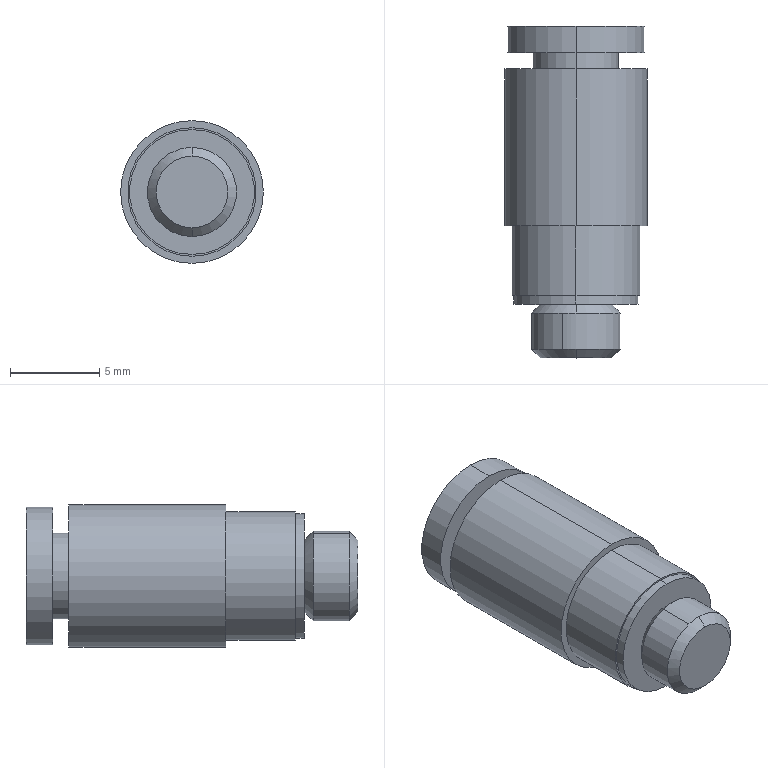Part | SolidWorks | features BaseBody 1 | 1 solid | 33 faces | box 8 x 18.6 x 8 mm | volume 570.386 mm3 | plane 15 | cylinder 14 | cone 4 | commonest cylinder face diameters 4 x2 4.8 x2 5 x2 7 x2 7.2 x2 7.7 x2
STEP:
#1=CARTESIAN_POINT('',(0.,15.6,3.85));
#2=VERTEX_POINT('',#1);
#3=CARTESIAN_POINT('',(0.,15.6,-3.85));
#4=VERTEX_POINT('',#3);
#5=CARTESIAN_POINT('',(0.,15.6,0.));
#6=DIRECTION('',(0.,-1.,0.));
#7=DIRECTION('',(0.,0.,-1.));
#8=AXIS2_PLACEMENT_3D('',#5,#6,#7);
#9=CIRCLE('',#8,3.85);
#10=EDGE_CURVE('',#2,#4,#9,.T.);
#11=ORIENTED_EDGE('',*,*,#10,.F.);
#12=CARTESIAN_POINT('',(0.,15.6,0.));
#13=DIRECTION('',(0.,-1.,0.));
#14=DIRECTION('',(0.,0.,-1.));
#15=AXIS2_PLACEMENT_3D('',#12,#13,#14);
#16=CIRCLE('',#15,3.85);
#17=EDGE_CURVE('',#4,#2,#16,.T.);
#18=ORIENTED_EDGE('',*,*,#17,.F.);
#19=EDGE_LOOP('',(#11,#18));
#20=FACE_OUTER_BOUND('',#19,.T.);
#21=CARTESIAN_POINT('',(0.,15.6,-2.));
#22=VERTEX_POINT('',#21);
#23=CARTESIAN_POINT('',(0.,15.6,2.));
#24=VERTEX_POINT('',#23);
#25=CARTESIAN_POINT('',(0.,15.6,0.));
#26=DIRECTION('',(0.,-1.,0.));
#27=DIRECTION('',(0.,0.,-1.));
#28=AXIS2_PLACEMENT_3D('',#25,#26,#27);
#29=CIRCLE('',#28,2.);
#30=EDGE_CURVE('',#22,#24,#29,.T.);
#31=ORIENTED_EDGE('',*,*,#30,.T.);
#32=CARTESIAN_POINT('',(0.,15.6,0.));
#33=DIRECTION('',(0.,-1.,0.));
#34=DIRECTION('',(0.,0.,-1.));
#35=AXIS2_PLACEMENT_3D('',#32,#33,#34);
#36=CIRCLE('',#35,2.);
#37=EDGE_CURVE('',#24,#22,#36,.T.);
#38=ORIENTED_EDGE('',*,*,#37,.T.);
#39=EDGE_LOOP('',(#31,#38));
#40=FACE_BOUND('',#39,.T.);
#41=CARTESIAN_POINT('',(0.,15.6,0.));
#42=DIRECTION('',(0.,-1.,0.));
#43=DIRECTION('',(0.,0.,-1.));
#44=AXIS2_PLACEMENT_3D('',#41,#42,#43);
#45=PLANE('',#44);
#46=ADVANCED_FACE('',(#20,#40),#45,.F.);
#47=CARTESIAN_POINT('',(0.,2.3,2.));
#48=VERTEX_POINT('',#47);
#49=CARTESIAN_POINT('',(0.,15.6,2.));
#50=DIRECTION('',(0.,-1.,0.));
#51=VECTOR('',#50,1000.);
#52=LINE('',#49,#51);
#53=EDGE_CURVE('',#24,#48,#52,.T.);
#54=ORIENTED_EDGE('',*,*,#53,.T.);
#55=CARTESIAN_POINT('',(0.,2.3,-2.));
#56=VERTEX_POINT('',#55);
#57=CARTESIAN_POINT('',(0.,2.3,0.));
#58=DIRECTION('',(0.,-1.,0.));
#59=DIRECTION('',(0.,0.,-1.));
#60=AXIS2_PLACEMENT_3D('',#57,#58,#59);
#61=CIRCLE('',#60,2.);
#62=EDGE_CURVE('',#48,#56,#61,.T.);
#63=ORIENTED_EDGE('',*,*,#62,.T.);
#64=CARTESIAN_POINT('',(0.,15.6,-2.));
#65=DIRECTION('',(0.,-1.,0.));
#66=VECTOR('',#65,1000.);
#67=LINE('',#64,#66);
#68=EDGE_CURVE('',#22,#56,#67,.T.);
#69=ORIENTED_EDGE('',*,*,#68,.F.);
#70=ORIENTED_EDGE('',*,*,#37,.F.);
#71=EDGE_LOOP('',(#54,#63,#69,#70));
#72=FACE_OUTER_BOUND('',#71,.T.);
#73=CARTESIAN_POINT('',(0.,2.3,0.));
#74=DIRECTION('',(0.,-1.,0.));
#75=DIRECTION('',(1.,0.,0.));
#76=AXIS2_PLACEMENT_3D('',#73,#74,#75);
#77=CYLINDRICAL_SURFACE('',#76,2.);
#78=ADVANCED_FACE('',(#72),#77,.F.);
#79=ORIENTED_EDGE('',*,*,#53,.F.);
#80=ORIENTED_EDGE('',*,*,#30,.F.);
#81=ORIENTED_EDGE('',*,*,#68,.T.);
#82=CARTESIAN_POINT('',(0.,2.3,0.));
#83=DIRECTION('',(0.,-1.,0.));
#84=DIRECTION('',(0.,0.,-1.));
#85=AXIS2_PLACEMENT_3D('',#82,#83,#84);
#86=CIRCLE('',#85,2.);
#87=EDGE_CURVE('',#56,#48,#86,.T.);
#88=ORIENTED_EDGE('',*,*,#87,.T.);
#89=EDGE_LOOP('',(#79,#80,#81,#88));
#90=FACE_OUTER_BOUND('',#89,.T.);
#91=CARTESIAN_POINT('',(0.,2.3,0.));
#92=DIRECTION('',(0.,-1.,0.));
#93=DIRECTION('',(-1.,0.,0.));
#94=AXIS2_PLACEMENT_3D('',#91,#92,#93);
#95=CYLINDRICAL_SURFACE('',#94,2.);
#96=ADVANCED_FACE('',(#90),#95,.F.);
#97=CARTESIAN_POINT('',(1.25,2.3,0.7217));
#98=VERTEX_POINT('',#97);
#99=CARTESIAN_POINT('',(1.25,2.3,-0.7217));
#100=VERTEX_POINT('',#99);
#101=CARTESIAN_POINT('',(1.25,2.3,0.));
#102=DIRECTION('',(0.,0.,-1.));
#103=VECTOR('',#102,1000.);
#104=LINE('',#101,#103);
#105=EDGE_CURVE('',#98,#100,#104,.T.);
#106=ORIENTED_EDGE('',*,*,#105,.F.);
#107=CARTESIAN_POINT('',(0.,2.3,1.443));
#108=VERTEX_POINT('',#107);
#109=CARTESIAN_POINT('',(2.125,2.3,0.2165));
#110=DIRECTION('',(0.866,0.,-0.5));
#111=VECTOR('',#110,1000.);
#112=LINE('',#109,#111);
#113=EDGE_CURVE('',#108,#98,#112,.T.);
#114=ORIENTED_EDGE('',*,*,#113,.F.);
#115=CARTESIAN_POINT('',(-1.25,2.3,0.7217));
#116=VERTEX_POINT('',#115);
#117=CARTESIAN_POINT('',(0.875,2.3,1.949));
#118=DIRECTION('',(0.866,0.,0.5));
#119=VECTOR('',#118,1000.);
#120=LINE('',#117,#119);
#121=EDGE_CURVE('',#116,#108,#120,.T.);
#122=ORIENTED_EDGE('',*,*,#121,.F.);
#123=CARTESIAN_POINT('',(-1.25,2.3,-0.7217));
#124=VERTEX_POINT('',#123);
#125=CARTESIAN_POINT('',(-1.25,2.3,0.));
#126=DIRECTION('',(0.,0.,1.));
#127=VECTOR('',#126,1000.);
#128=LINE('',#125,#127);
#129=EDGE_CURVE('',#124,#116,#128,.T.);
#130=ORIENTED_EDGE('',*,*,#129,.F.);
#131=CARTESIAN_POINT('',(0.,2.3,-1.443));
#132=VERTEX_POINT('',#131);
#133=CARTESIAN_POINT('',(0.875,2.3,-1.949));
#134=DIRECTION('',(-0.866,0.,0.5));
#135=VECTOR('',#134,1000.);
#136=LINE('',#133,#135);
#137=EDGE_CURVE('',#132,#124,#136,.T.);
#138=ORIENTED_EDGE('',*,*,#137,.F.);
#139=CARTESIAN_POINT('',(2.125,2.3,-0.2165));
#140=DIRECTION('',(-0.866,0.,-0.5));
#141=VECTOR('',#140,1000.);
#142=LINE('',#139,#141);
#143=EDGE_CURVE('',#100,#132,#142,.T.);
#144=ORIENTED_EDGE('',*,*,#143,.F.);
#145=EDGE_LOOP('',(#106,#114,#122,#130,#138,#144));
#146=FACE_BOUND('',#145,.T.);
#147=ORIENTED_EDGE('',*,*,#62,.F.);
#148=ORIENTED_EDGE('',*,*,#87,.F.);
#149=EDGE_LOOP('',(#147,#148));
#150=FACE_OUTER_BOUND('',#149,.T.);
#151=CARTESIAN_POINT('',(2.,2.3,0.));
#152=DIRECTION('',(0.,1.,0.));
#153=DIRECTION('',(0.,0.,1.));
#154=AXIS2_PLACEMENT_3D('',#151,#152,#153);
#155=PLANE('',#154);
#156=ADVANCED_FACE('',(#146,#150),#155,.T.);
#157=ORIENTED_EDGE('',*,*,#143,.T.);
#158=CARTESIAN_POINT('',(0.,-2.2,-1.443));
#159=VERTEX_POINT('',#158);
#160=CARTESIAN_POINT('',(0.,-2.2,-1.443));
#161=DIRECTION('',(0.,1.,0.));
#162=VECTOR('',#161,1000.);
#163=LINE('',#160,#162);
#164=EDGE_CURVE('',#159,#132,#163,.T.);
#165=ORIENTED_EDGE('',*,*,#164,.F.);
#166=CARTESIAN_POINT('',(1.25,-2.2,-0.7217));
#167=VERTEX_POINT('',#166);
#168=CARTESIAN_POINT('',(1.25,-2.2,-0.7217));
#169=DIRECTION('',(-0.866,0.,-0.5));
#170=VECTOR('',#169,1000.);
#171=LINE('',#168,#170);
#172=EDGE_CURVE('',#167,#159,#171,.T.);
#173=ORIENTED_EDGE('',*,*,#172,.F.);
#174=CARTESIAN_POINT('',(1.25,-2.2,-0.7217));
#175=DIRECTION('',(0.,1.,0.));
#176=VECTOR('',#175,1000.);
#177=LINE('',#174,#176);
#178=EDGE_CURVE('',#167,#100,#177,.T.);
#179=ORIENTED_EDGE('',*,*,#178,.T.);
#180=EDGE_LOOP('',(#157,#165,#173,#179));
#181=FACE_OUTER_BOUND('',#180,.T.);
#182=CARTESIAN_POINT('',(1.25,-2.2,-0.7217));
#183=DIRECTION('',(0.5,0.,-0.866));
#184=DIRECTION('',(-0.866,0.,-0.5));
#185=AXIS2_PLACEMENT_3D('',#182,#183,#184);
#186=PLANE('',#185);
#187=ADVANCED_FACE('',(#181),#186,.F.);
#188=CARTESIAN_POINT('',(1.25,-2.2,0.7217));
#189=VERTEX_POINT('',#188);
#190=CARTESIAN_POINT('',(1.25,-2.2,0.7217));
#191=DIRECTION('',(0.,1.,0.));
#192=VECTOR('',#191,1000.);
#193=LINE('',#190,#192);
#194=EDGE_CURVE('',#189,#98,#193,.T.);
#195=ORIENTED_EDGE('',*,*,#194,.T.);
#196=ORIENTED_EDGE('',*,*,#105,.T.);
#197=ORIENTED_EDGE('',*,*,#178,.F.);
#198=CARTESIAN_POINT('',(1.25,-2.2,0.7217));
#199=DIRECTION('',(0.,0.,-1.));
#200=VECTOR('',#199,1000.);
#201=LINE('',#198,#200);
#202=EDGE_CURVE('',#189,#167,#201,.T.);
#203=ORIENTED_EDGE('',*,*,#202,.F.);
#204=EDGE_LOOP('',(#195,#196,#197,#203));
#205=FACE_OUTER_BOUND('',#204,.T.);
#206=CARTESIAN_POINT('',(1.25,-2.2,0.7217));
#207=DIRECTION('',(1.,0.,0.));
#208=DIRECTION('',(0.,0.,-1.));
#209=AXIS2_PLACEMENT_3D('',#206,#207,#208);
#210=PLANE('',#209);
#211=ADVANCED_FACE('',(#205),#210,.F.);
#212=CARTESIAN_POINT('',(-1.25,-2.2,-0.7217));
#213=VERTEX_POINT('',#212);
#214=CARTESIAN_POINT('',(-1.25,-2.2,0.7217));
#215=VERTEX_POINT('',#214);
#216=CARTESIAN_POINT('',(-1.25,-2.2,-0.7217));
#217=DIRECTION('',(0.,0.,1.));
#218=VECTOR('',#217,1000.);
#219=LINE('',#216,#218);
#220=EDGE_CURVE('',#213,#215,#219,.T.);
#221=ORIENTED_EDGE('',*,*,#220,.T.);
#222=CARTESIAN_POINT('',(0.,-2.2,1.443));
#223=VERTEX_POINT('',#222);
#224=CARTESIAN_POINT('',(-1.25,-2.2,0.7217));
#225=DIRECTION('',(0.866,0.,0.5));
#226=VECTOR('',#225,1000.);
#227=LINE('',#224,#226);
#228=EDGE_CURVE('',#215,#223,#227,.T.);
#229=ORIENTED_EDGE('',*,*,#228,.T.);
#230=CARTESIAN_POINT('',(0.,-2.2,1.443));
#231=DIRECTION('',(0.866,0.,-0.5));
#232=VECTOR('',#231,1000.);
#233=LINE('',#230,#232);
#234=EDGE_CURVE('',#223,#189,#233,.T.);
#235=ORIENTED_EDGE('',*,*,#234,.T.);
#236=ORIENTED_EDGE('',*,*,#202,.T.);
#237=ORIENTED_EDGE('',*,*,#172,.T.);
#238=CARTESIAN_POINT('',(0.,-2.2,-1.443));
#239=DIRECTION('',(-0.866,0.,0.5));
#240=VECTOR('',#239,1000.);
#241=LINE('',#238,#240);
#242=EDGE_CURVE('',#159,#213,#241,.T.);
#243=ORIENTED_EDGE('',*,*,#242,.T.);
#244=EDGE_LOOP('',(#221,#229,#235,#236,#237,#243));
#245=FACE_OUTER_BOUND('',#244,.T.);
#246=CARTESIAN_POINT('',(0.,-2.2,0.));
#247=DIRECTION('',(0.,1.,0.));
#248=DIRECTION('',(0.,0.,1.));
#249=AXIS2_PLACEMENT_3D('',#246,#247,#248);
#250=PLANE('',#249);
#251=ADVANCED_FACE('',(#245),#250,.T.);
#252=ORIENTED_EDGE('',*,*,#137,.T.);
#253=CARTESIAN_POINT('',(-1.25,-2.2,-0.7217));
#254=DIRECTION('',(0.,1.,0.));
#255=VECTOR('',#254,1000.);
#256=LINE('',#253,#255);
#257=EDGE_CURVE('',#213,#124,#256,.T.);
#258=ORIENTED_EDGE('',*,*,#257,.F.);
#259=ORIENTED_EDGE('',*,*,#242,.F.);
#260=ORIENTED_EDGE('',*,*,#164,.T.);
#261=EDGE_LOOP('',(#252,#258,#259,#260));
#262=FACE_OUTER_BOUND('',#261,.T.);
#263=CARTESIAN_POINT('',(0.,-2.2,-1.443));
#264=DIRECTION('',(-0.5,0.,-0.866));
#265=DIRECTION('',(-0.866,0.,0.5));
#266=AXIS2_PLACEMENT_3D('',#263,#264,#265);
#267=PLANE('',#266);
#268=ADVANCED_FACE('',(#262),#267,.F.);
#269=ORIENTED_EDGE('',*,*,#129,.T.);
#270=CARTESIAN_POINT('',(-1.25,-2.2,0.7217));
#271=DIRECTION('',(0.,1.,0.));
#272=VECTOR('',#271,1000.);
#273=LINE('',#270,#272);
#274=EDGE_CURVE('',#215,#116,#273,.T.);
#275=ORIENTED_EDGE('',*,*,#274,.F.);
#276=ORIENTED_EDGE('',*,*,#220,.F.);
#277=ORIENTED_EDGE('',*,*,#257,.T.);
#278=EDGE_LOOP('',(#269,#275,#276,#277));
#279=FACE_OUTER_BOUND('',#278,.T.);
#280=CARTESIAN_POINT('',(-1.25,-2.2,-0.7217));
#281=DIRECTION('',(-1.,0.,0.));
#282=DIRECTION('',(0.,0.,1.));
#283=AXIS2_PLACEMENT_3D('',#280,#281,#282);
#284=PLANE('',#283);
#285=ADVANCED_FACE('',(#279),#284,.F.);
#286=ORIENTED_EDGE('',*,*,#121,.T.);
#287=CARTESIAN_POINT('',(0.,-2.2,1.443));
#288=DIRECTION('',(0.,1.,0.));
#289=VECTOR('',#288,1000.);
#290=LINE('',#287,#289);
#291=EDGE_CURVE('',#223,#108,#290,.T.);
#292=ORIENTED_EDGE('',*,*,#291,.F.);
#293=ORIENTED_EDGE('',*,*,#228,.F.);
#294=ORIENTED_EDGE('',*,*,#274,.T.);
#295=EDGE_LOOP('',(#286,#292,#293,#294));
#296=FACE_OUTER_BOUND('',#295,.T.);
#297=CARTESIAN_POINT('',(-1.25,-2.2,0.7217));
#298=DIRECTION('',(-0.5,0.,0.866));
#299=DIRECTION('',(0.866,0.,0.5));
#300=AXIS2_PLACEMENT_3D('',#297,#298,#299);
#301=PLANE('',#300);
#302=ADVANCED_FACE('',(#296),#301,.F.);
#303=ORIENTED_EDGE('',*,*,#113,.T.);
#304=ORIENTED_EDGE('',*,*,#194,.F.);
#305=ORIENTED_EDGE('',*,*,#234,.F.);
#306=ORIENTED_EDGE('',*,*,#291,.T.);
#307=EDGE_LOOP('',(#303,#304,#305,#306));
#308=FACE_OUTER_BOUND('',#307,.T.);
#309=CARTESIAN_POINT('',(0.,-2.2,1.443));
#310=DIRECTION('',(0.5,0.,0.866));
#311=DIRECTION('',(0.866,0.,-0.5));
#312=AXIS2_PLACEMENT_3D('',#309,#310,#311);
#313=PLANE('',#312);
#314=ADVANCED_FACE('',(#308),#313,.F.);
#315=CARTESIAN_POINT('',(0.,14.1,3.85));
#316=VERTEX_POINT('',#315);
#317=CARTESIAN_POINT('',(0.,15.6,3.85));
#318=DIRECTION('',(0.,-1.,0.));
#319=VECTOR('',#318,1000.);
#320=LINE('',#317,#319);
#321=EDGE_CURVE('',#2,#316,#320,.T.);
#322=ORIENTED_EDGE('',*,*,#321,.T.);
#323=CARTESIAN_POINT('',(0.,14.1,-3.85));
#324=VERTEX_POINT('',#323);
#325=CARTESIAN_POINT('',(0.,14.1,0.));
#326=DIRECTION('',(0.,-1.,0.));
#327=DIRECTION('',(0.,0.,-1.));
#328=AXIS2_PLACEMENT_3D('',#325,#326,#327);
#329=CIRCLE('',#328,3.85);
#330=EDGE_CURVE('',#324,#316,#329,.T.);
#331=ORIENTED_EDGE('',*,*,#330,.F.);
#332=CARTESIAN_POINT('',(0.,15.6,-3.85));
#333=DIRECTION('',(0.,-1.,0.));
#334=VECTOR('',#333,1000.);
#335=LINE('',#332,#334);
#336=EDGE_CURVE('',#4,#324,#335,.T.);
#337=ORIENTED_EDGE('',*,*,#336,.F.);
#338=ORIENTED_EDGE('',*,*,#17,.T.);
#339=EDGE_LOOP('',(#322,#331,#337,#338));
#340=FACE_OUTER_BOUND('',#339,.T.);
#341=CARTESIAN_POINT('',(0.,-3.,0.));
#342=DIRECTION('',(0.,-1.,0.));
#343=DIRECTION('',(-1.,0.,0.));
#344=AXIS2_PLACEMENT_3D('',#341,#342,#343);
#345=CYLINDRICAL_SURFACE('',#344,3.85);
#346=ADVANCED_FACE('',(#340),#345,.T.);
#347=ORIENTED_EDGE('',*,*,#321,.F.);
#348=ORIENTED_EDGE('',*,*,#10,.T.);
#349=ORIENTED_EDGE('',*,*,#336,.T.);
#350=CARTESIAN_POINT('',(0.,14.1,0.));
#351=DIRECTION('',(0.,-1.,0.));
#352=DIRECTION('',(0.,0.,-1.));
#353=AXIS2_PLACEMENT_3D('',#350,#351,#352);
#354=CIRCLE('',#353,3.85);
#355=EDGE_CURVE('',#316,#324,#354,.T.);
#356=ORIENTED_EDGE('',*,*,#355,.F.);
#357=EDGE_LOOP('',(#347,#348,#349,#356));
#358=FACE_OUTER_BOUND('',#357,.T.);
#359=CARTESIAN_POINT('',(0.,-3.,0.));
#360=DIRECTION('',(0.,-1.,0.));
#361=DIRECTION('',(1.,0.,0.));
#362=AXIS2_PLACEMENT_3D('',#359,#360,#361);
#363=CYLINDRICAL_SURFACE('',#362,3.85);
#364=ADVANCED_FACE('',(#358),#363,.T.);
#365=CARTESIAN_POINT('',(0.,14.1,2.4));
#366=VERTEX_POINT('',#365);
#367=CARTESIAN_POINT('',(0.,14.1,-2.4));
#368=VERTEX_POINT('',#367);
#369=CARTESIAN_POINT('',(0.,14.1,0.));
#370=DIRECTION('',(0.,-1.,0.));
#371=DIRECTION('',(0.,0.,-1.));
#372=AXIS2_PLACEMENT_3D('',#369,#370,#371);
#373=CIRCLE('',#372,2.4);
#374=EDGE_CURVE('',#366,#368,#373,.T.);
#375=ORIENTED_EDGE('',*,*,#374,.F.);
#376=CARTESIAN_POINT('',(0.,14.1,0.));
#377=DIRECTION('',(0.,-1.,0.));
#378=DIRECTION('',(0.,0.,-1.));
#379=AXIS2_PLACEMENT_3D('',#376,#377,#378);
#380=CIRCLE('',#379,2.4);
#381=EDGE_CURVE('',#368,#366,#380,.T.);
#382=ORIENTED_EDGE('',*,*,#381,.F.);
#383=EDGE_LOOP('',(#375,#382));
#384=FACE_BOUND('',#383,.T.);
#385=ORIENTED_EDGE('',*,*,#330,.T.);
#386=ORIENTED_EDGE('',*,*,#355,.T.);
#387=EDGE_LOOP('',(#385,#386));
#388=FACE_OUTER_BOUND('',#387,.T.);
#389=CARTESIAN_POINT('',(3.85,14.1,0.));
#390=DIRECTION('',(0.,1.,0.));
#391=DIRECTION('',(0.,0.,1.));
#392=AXIS2_PLACEMENT_3D('',#389,#390,#391);
#393=PLANE('',#392);
#394=ADVANCED_FACE('',(#384,#388),#393,.F.);
#395=CARTESIAN_POINT('',(0.,13.2,2.4));
#396=VERTEX_POINT('',#395);
#397=CARTESIAN_POINT('',(0.,14.1,2.4));
#398=DIRECTION('',(0.,-1.,0.));
#399=VECTOR('',#398,1000.);
#400=LINE('',#397,#399);
#401=EDGE_CURVE('',#366,#396,#400,.T.);
#402=ORIENTED_EDGE('',*,*,#401,.T.);
#403=CARTESIAN_POINT('',(0.,13.2,-2.4));
#404=VERTEX_POINT('',#403);
#405=CARTESIAN_POINT('',(0.,13.2,0.));
#406=DIRECTION('',(0.,-1.,0.));
#407=DIRECTION('',(0.,0.,-1.));
#408=AXIS2_PLACEMENT_3D('',#405,#406,#407);
#409=CIRCLE('',#408,2.4);
#410=EDGE_CURVE('',#404,#396,#409,.T.);
#411=ORIENTED_EDGE('',*,*,#410,.F.);
#412=CARTESIAN_POINT('',(0.,14.1,-2.4));
#413=DIRECTION('',(0.,-1.,0.));
#414=VECTOR('',#413,1000.);
#415=LINE('',#412,#414);
#416=EDGE_CURVE('',#368,#404,#415,.T.);
#417=ORIENTED_EDGE('',*,*,#416,.F.);
#418=ORIENTED_EDGE('',*,*,#381,.T.);
#419=EDGE_LOOP('',(#402,#411,#417,#418));
#420=FACE_OUTER_BOUND('',#419,.T.);
#421=CARTESIAN_POINT('',(0.,-3.,0.));
#422=DIRECTION('',(0.,-1.,0.));
#423=DIRECTION('',(-1.,0.,0.));
#424=AXIS2_PLACEMENT_3D('',#421,#422,#423);
#425=CYLINDRICAL_SURFACE('',#424,2.4);
#426=ADVANCED_FACE('',(#420),#425,.T.);
#427=ORIENTED_EDGE('',*,*,#401,.F.);
#428=ORIENTED_EDGE('',*,*,#374,.T.);
#429=ORIENTED_EDGE('',*,*,#416,.T.);
#430=CARTESIAN_POINT('',(0.,13.2,0.));
#431=DIRECTION('',(0.,-1.,0.));
#432=DIRECTION('',(0.,0.,-1.));
#433=AXIS2_PLACEMENT_3D('',#430,#431,#432);
#434=CIRCLE('',#433,2.4);
#435=EDGE_CURVE('',#396,#404,#434,.T.);
#436=ORIENTED_EDGE('',*,*,#435,.F.);
#437=EDGE_LOOP('',(#427,#428,#429,#436));
#438=FACE_OUTER_BOUND('',#437,.T.);
#439=CARTESIAN_POINT('',(0.,-3.,0.));
#440=DIRECTION('',(0.,-1.,0.));
#441=DIRECTION('',(1.,0.,0.));
#442=AXIS2_PLACEMENT_3D('',#439,#440,#441);
#443=CYLINDRICAL_SURFACE('',#442,2.4);
#444=ADVANCED_FACE('',(#438),#443,.T.);
#445=CARTESIAN_POINT('',(0.,13.2,4.));
#446=VERTEX_POINT('',#445);
#447=CARTESIAN_POINT('',(0.,13.2,-4.));
#448=VERTEX_POINT('',#447);
#449=CARTESIAN_POINT('',(0.,13.2,0.));
#450=DIRECTION('',(0.,-1.,0.));
#451=DIRECTION('',(0.,0.,-1.));
#452=AXIS2_PLACEMENT_3D('',#449,#450,#451);
#453=CIRCLE('',#452,4.);
#454=EDGE_CURVE('',#446,#448,#453,.T.);
#455=ORIENTED_EDGE('',*,*,#454,.F.);
#456=CARTESIAN_POINT('',(0.,13.2,0.));
#457=DIRECTION('',(0.,-1.,0.));
#458=DIRECTION('',(0.,0.,-1.));
#459=AXIS2_PLACEMENT_3D('',#456,#457,#458);
#460=CIRCLE('',#459,4.);
#461=EDGE_CURVE('',#448,#446,#460,.T.);
#462=ORIENTED_EDGE('',*,*,#461,.F.);
#463=EDGE_LOOP('',(#455,#462));
#464=FACE_OUTER_BOUND('',#463,.T.);
#465=ORIENTED_EDGE('',*,*,#410,.T.);
#466=ORIENTED_EDGE('',*,*,#435,.T.);
#467=EDGE_LOOP('',(#465,#466));
#468=FACE_BOUND('',#467,.T.);
#469=CARTESIAN_POINT('',(2.4,13.2,0.));
#470=DIRECTION('',(0.,-1.,0.));
#471=DIRECTION('',(0.,0.,-1.));
#472=AXIS2_PLACEMENT_3D('',#469,#470,#471);
#473=PLANE('',#472);
#474=ADVANCED_FACE('',(#464,#468),#473,.F.);
#475=CARTESIAN_POINT('',(0.,4.4,4.));
#476=VERTEX_POINT('',#475);
#477=CARTESIAN_POINT('',(0.,13.2,4.));
#478=DIRECTION('',(0.,-1.,0.));
#479=VECTOR('',#478,1000.);
#480=LINE('',#477,#479);
#481=EDGE_CURVE('',#446,#476,#480,.T.);
#482=ORIENTED_EDGE('',*,*,#481,.T.);
#483=CARTESIAN_POINT('',(0.,4.4,-4.));
#484=VERTEX_POINT('',#483);
#485=CARTESIAN_POINT('',(0.,4.4,0.));
#486=DIRECTION('',(0.,1.,0.));
#487=DIRECTION('',(0.,0.,1.));
#488=AXIS2_PLACEMENT_3D('',#485,#486,#487);
#489=CIRCLE('',#488,4.);
#490=EDGE_CURVE('',#476,#484,#489,.T.);
#491=ORIENTED_EDGE('',*,*,#490,.T.);
#492=CARTESIAN_POINT('',(0.,13.2,-4.));
#493=DIRECTION('',(0.,-1.,0.));
#494=VECTOR('',#493,1000.);
#495=LINE('',#492,#494);
#496=EDGE_CURVE('',#448,#484,#495,.T.);
#497=ORIENTED_EDGE('',*,*,#496,.F.);
#498=ORIENTED_EDGE('',*,*,#461,.T.);
#499=EDGE_LOOP('',(#482,#491,#497,#498));
#500=FACE_OUTER_BOUND('',#499,.T.);
#501=CARTESIAN_POINT('',(0.,-3.,0.));
#502=DIRECTION('',(0.,-1.,0.));
#503=DIRECTION('',(-1.,0.,0.));
#504=AXIS2_PLACEMENT_3D('',#501,#502,#503);
#505=CYLINDRICAL_SURFACE('',#504,4.);
#506=ADVANCED_FACE('',(#500),#505,.T.);
#507=ORIENTED_EDGE('',*,*,#481,.F.);
#508=ORIENTED_EDGE('',*,*,#454,.T.);
#509=ORIENTED_EDGE('',*,*,#496,.T.);
#510=CARTESIAN_POINT('',(0.,4.4,0.));
#511=DIRECTION('',(0.,1.,0.));
#512=DIRECTION('',(0.,0.,1.));
#513=AXIS2_PLACEMENT_3D('',#510,#511,#512);
#514=CIRCLE('',#513,4.);
#515=EDGE_CURVE('',#484,#476,#514,.T.);
#516=ORIENTED_EDGE('',*,*,#515,.T.);
#517=EDGE_LOOP('',(#507,#508,#509,#516));
#518=FACE_OUTER_BOUND('',#517,.T.);
#519=CARTESIAN_POINT('',(0.,-3.,0.));
#520=DIRECTION('',(0.,-1.,0.));
#521=DIRECTION('',(1.,0.,0.));
#522=AXIS2_PLACEMENT_3D('',#519,#520,#521);
#523=CYLINDRICAL_SURFACE('',#522,4.);
#524=ADVANCED_FACE('',(#518),#523,.T.);
#525=CARTESIAN_POINT('',(0.,4.4,3.6));
#526=VERTEX_POINT('',#525);
#527=CARTESIAN_POINT('',(0.,4.4,-3.6));
#528=VERTEX_POINT('',#527);
#529=CARTESIAN_POINT('',(0.,4.4,0.));
#530=DIRECTION('',(0.,-1.,0.));
#531=DIRECTION('',(0.,0.,-1.));
#532=AXIS2_PLACEMENT_3D('',#529,#530,#531);
#533=CIRCLE('',#532,3.6);
#534=EDGE_CURVE('',#526,#528,#533,.T.);
#535=ORIENTED_EDGE('',*,*,#534,.F.);
#536=CARTESIAN_POINT('',(0.,4.4,0.));
#537=DIRECTION('',(0.,-1.,0.));
#538=DIRECTION('',(0.,0.,-1.));
#539=AXIS2_PLACEMENT_3D('',#536,#537,#538);
#540=CIRCLE('',#539,3.6);
#541=EDGE_CURVE('',#528,#526,#540,.T.);
#542=ORIENTED_EDGE('',*,*,#541,.F.);
#543=EDGE_LOOP('',(#535,#542));
#544=FACE_BOUND('',#543,.T.);
#545=ORIENTED_EDGE('',*,*,#515,.F.);
#546=ORIENTED_EDGE('',*,*,#490,.F.);
#547=EDGE_LOOP('',(#545,#546));
#548=FACE_OUTER_BOUND('',#547,.T.);
#549=CARTESIAN_POINT('',(6.5,4.4,0.));
#550=DIRECTION('',(0.,1.,0.));
#551=DIRECTION('',(0.,0.,1.));
#552=AXIS2_PLACEMENT_3D('',#549,#550,#551);
#553=PLANE('',#552);
#554=ADVANCED_FACE('',(#544,#548),#553,.F.);
#555=CARTESIAN_POINT('',(0.,0.5,3.6));
#556=VERTEX_POINT('',#555);
#557=CARTESIAN_POINT('',(0.,4.4,3.6));
#558=DIRECTION('',(0.,-1.,0.));
#559=VECTOR('',#558,1000.);
#560=LINE('',#557,#559);
#561=EDGE_CURVE('',#526,#556,#560,.T.);
#562=ORIENTED_EDGE('',*,*,#561,.T.);
#563=CARTESIAN_POINT('',(0.,0.5,-3.6));
#564=VERTEX_POINT('',#563);
#565=CARTESIAN_POINT('',(0.,0.5,0.));
#566=DIRECTION('',(0.,-1.,0.));
#567=DIRECTION('',(0.,0.,-1.));
#568=AXIS2_PLACEMENT_3D('',#565,#566,#567);
#569=CIRCLE('',#568,3.6);
#570=EDGE_CURVE('',#564,#556,#569,.T.);
#571=ORIENTED_EDGE('',*,*,#570,.F.);
#572=CARTESIAN_POINT('',(0.,4.4,-3.6));
#573=DIRECTION('',(0.,-1.,0.));
#574=VECTOR('',#573,1000.);
#575=LINE('',#572,#574);
#576=EDGE_CURVE('',#528,#564,#575,.T.);
#577=ORIENTED_EDGE('',*,*,#576,.F.);
#578=ORIENTED_EDGE('',*,*,#541,.T.);
#579=EDGE_LOOP('',(#562,#571,#577,#578));
#580=FACE_OUTER_BOUND('',#579,.T.);
#581=CARTESIAN_POINT('',(0.,0.,0.));
#582=DIRECTION('',(0.,-1.,0.));
#583=DIRECTION('',(-1.,0.,0.));
#584=AXIS2_PLACEMENT_3D('',#581,#582,#583);
#585=CYLINDRICAL_SURFACE('',#584,3.6);
#586=ADVANCED_FACE('',(#580),#585,.T.);
#587=ORIENTED_EDGE('',*,*,#561,.F.);
#588=ORIENTED_EDGE('',*,*,#534,.T.);
#589=ORIENTED_EDGE('',*,*,#576,.T.);
#590=CARTESIAN_POINT('',(0.,0.5,0.));
#591=DIRECTION('',(0.,-1.,0.));
#592=DIRECTION('',(0.,0.,-1.));
#593=AXIS2_PLACEMENT_3D('',#590,#591,#592);
#594=CIRCLE('',#593,3.6);
#595=EDGE_CURVE('',#556,#564,#594,.T.);
#596=ORIENTED_EDGE('',*,*,#595,.F.);
#597=EDGE_LOOP('',(#587,#588,#589,#596));
#598=FACE_OUTER_BOUND('',#597,.T.);
#599=CARTESIAN_POINT('',(0.,0.,0.));
#600=DIRECTION('',(0.,-1.,0.));
#601=DIRECTION('',(1.,0.,0.));
#602=AXIS2_PLACEMENT_3D('',#599,#600,#601);
#603=CYLINDRICAL_SURFACE('',#602,3.6);
#604=ADVANCED_FACE('',(#598),#603,.T.);
#605=CARTESIAN_POINT('',(0.,0.5,3.5));
#606=VERTEX_POINT('',#605);
#607=CARTESIAN_POINT('',(0.,0.5,-3.5));
#608=VERTEX_POINT('',#607);
#609=CARTESIAN_POINT('',(0.,0.5,0.));
#610=DIRECTION('',(0.,-1.,0.));
#611=DIRECTION('',(0.,0.,-1.));
#612=AXIS2_PLACEMENT_3D('',#609,#610,#611);
#613=CIRCLE('',#612,3.5);
#614=EDGE_CURVE('',#606,#608,#613,.T.);
#615=ORIENTED_EDGE('',*,*,#614,.F.);
#616=CARTESIAN_POINT('',(0.,0.5,0.));
#617=DIRECTION('',(0.,-1.,0.));
#618=DIRECTION('',(0.,0.,-1.));
#619=AXIS2_PLACEMENT_3D('',#616,#617,#618);
#620=CIRCLE('',#619,3.5);
#621=EDGE_CURVE('',#608,#606,#620,.T.);
#622=ORIENTED_EDGE('',*,*,#621,.F.);
#623=EDGE_LOOP('',(#615,#622));
#624=FACE_BOUND('',#623,.T.);
#625=ORIENTED_EDGE('',*,*,#570,.T.);
#626=ORIENTED_EDGE('',*,*,#595,.T.);
#627=EDGE_LOOP('',(#625,#626));
#628=FACE_OUTER_BOUND('',#627,.T.);
#629=CARTESIAN_POINT('',(3.6,0.5,0.));
#630=DIRECTION('',(0.,1.,0.));
#631=DIRECTION('',(0.,0.,1.));
#632=AXIS2_PLACEMENT_3D('',#629,#630,#631);
#633=PLANE('',#632);
#634=ADVANCED_FACE('',(#624,#628),#633,.F.);
#635=CARTESIAN_POINT('',(0.,0.,3.5));
#636=VERTEX_POINT('',#635);
#637=CARTESIAN_POINT('',(0.,0.5,3.5));
#638=DIRECTION('',(0.,-1.,0.));
#639=VECTOR('',#638,1000.);
#640=LINE('',#637,#639);
#641=EDGE_CURVE('',#606,#636,#640,.T.);
#642=ORIENTED_EDGE('',*,*,#641,.T.);
#643=CARTESIAN_POINT('',(0.,0.,-3.5));
#644=VERTEX_POINT('',#643);
#645=CARTESIAN_POINT('',(0.,0.,0.));
#646=DIRECTION('',(0.,-1.,0.));
#647=DIRECTION('',(0.,0.,-1.));
#648=AXIS2_PLACEMENT_3D('',#645,#646,#647);
#649=CIRCLE('',#648,3.5);
#650=EDGE_CURVE('',#644,#636,#649,.T.);
#651=ORIENTED_EDGE('',*,*,#650,.F.);
#652=CARTESIAN_POINT('',(0.,0.5,-3.5));
#653=DIRECTION('',(0.,-1.,0.));
#654=VECTOR('',#653,1000.);
#655=LINE('',#652,#654);
#656=EDGE_CURVE('',#608,#644,#655,.T.);
#657=ORIENTED_EDGE('',*,*,#656,.F.);
#658=ORIENTED_EDGE('',*,*,#621,.T.);
#659=EDGE_LOOP('',(#642,#651,#657,#658));
#660=FACE_OUTER_BOUND('',#659,.T.);
#661=CARTESIAN_POINT('',(0.,0.,0.));
#662=DIRECTION('',(0.,-1.,0.));
#663=DIRECTION('',(-1.,0.,0.));
#664=AXIS2_PLACEMENT_3D('',#661,#662,#663);
#665=CYLINDRICAL_SURFACE('',#664,3.5);
#666=ADVANCED_FACE('',(#660),#665,.T.);
#667=ORIENTED_EDGE('',*,*,#641,.F.);
#668=ORIENTED_EDGE('',*,*,#614,.T.);
#669=ORIENTED_EDGE('',*,*,#656,.T.);
#670=CARTESIAN_POINT('',(0.,0.,0.));
#671=DIRECTION('',(0.,-1.,0.));
#672=DIRECTION('',(0.,0.,-1.));
#673=AXIS2_PLACEMENT_3D('',#670,#671,#672);
#674=CIRCLE('',#673,3.5);
#675=EDGE_CURVE('',#636,#644,#674,.T.);
#676=ORIENTED_EDGE('',*,*,#675,.F.);
#677=EDGE_LOOP('',(#667,#668,#669,#676));
#678=FACE_OUTER_BOUND('',#677,.T.);
#679=CARTESIAN_POINT('',(0.,0.,0.));
#680=DIRECTION('',(0.,-1.,0.));
#681=DIRECTION('',(1.,0.,0.));
#682=AXIS2_PLACEMENT_3D('',#679,#680,#681);
#683=CYLINDRICAL_SURFACE('',#682,3.5);
#684=ADVANCED_FACE('',(#678),#683,.T.);
#685=CARTESIAN_POINT('',(0.,0.,2.01));
#686=VERTEX_POINT('',#685);
#687=CARTESIAN_POINT('',(0.,0.,-2.01));
#688=VERTEX_POINT('',#687);
#689=CARTESIAN_POINT('',(0.,0.,0.));
#690=DIRECTION('',(0.,-1.,0.));
#691=DIRECTION('',(0.,0.,-1.));
#692=AXIS2_PLACEMENT_3D('',#689,#690,#691);
#693=CIRCLE('',#692,2.01);
#694=EDGE_CURVE('',#686,#688,#693,.T.);
#695=ORIENTED_EDGE('',*,*,#694,.F.);
#696=CARTESIAN_POINT('',(0.,0.,0.));
#697=DIRECTION('',(0.,-1.,0.));
#698=DIRECTION('',(0.,0.,-1.));
#699=AXIS2_PLACEMENT_3D('',#696,#697,#698);
#700=CIRCLE('',#699,2.01);
#701=EDGE_CURVE('',#688,#686,#700,.T.);
#702=ORIENTED_EDGE('',*,*,#701,.F.);
#703=EDGE_LOOP('',(#695,#702));
#704=FACE_BOUND('',#703,.T.);
#705=ORIENTED_EDGE('',*,*,#650,.T.);
#706=ORIENTED_EDGE('',*,*,#675,.T.);
#707=EDGE_LOOP('',(#705,#706));
#708=FACE_OUTER_BOUND('',#707,.T.);
#709=CARTESIAN_POINT('',(4.,0.,0.));
#710=DIRECTION('',(0.,1.,0.));
#711=DIRECTION('',(0.,0.,1.));
#712=AXIS2_PLACEMENT_3D('',#709,#710,#711);
#713=PLANE('',#712);
#714=ADVANCED_FACE('',(#704,#708),#713,.F.);
#715=CARTESIAN_POINT('',(0.,-0.4905,2.5));
#716=VERTEX_POINT('',#715);
#717=CARTESIAN_POINT('',(0.,0.,2.01));
#718=DIRECTION('',(0.,-0.7071,0.7071));
#719=VECTOR('',#718,1000.);
#720=LINE('',#717,#719);
#721=EDGE_CURVE('',#686,#716,#720,.T.);
#722=ORIENTED_EDGE('',*,*,#721,.T.);
#723=CARTESIAN_POINT('',(0.,-0.4905,-2.5));
#724=VERTEX_POINT('',#723);
#725=CARTESIAN_POINT('',(0.,-0.4905,0.));
#726=DIRECTION('',(0.,-1.,0.));
#727=DIRECTION('',(0.,0.,-1.));
#728=AXIS2_PLACEMENT_3D('',#725,#726,#727);
#729=CIRCLE('',#728,2.5);
#730=EDGE_CURVE('',#724,#716,#729,.T.);
#731=ORIENTED_EDGE('',*,*,#730,.F.);
#732=CARTESIAN_POINT('',(0.,0.,-2.01));
#733=DIRECTION('',(0.,-0.7071,-0.7071));
#734=VECTOR('',#733,1000.);
#735=LINE('',#732,#734);
#736=EDGE_CURVE('',#688,#724,#735,.T.);
#737=ORIENTED_EDGE('',*,*,#736,.F.);
#738=ORIENTED_EDGE('',*,*,#701,.T.);
#739=EDGE_LOOP('',(#722,#731,#737,#738));
#740=FACE_OUTER_BOUND('',#739,.T.);
#741=CARTESIAN_POINT('',(0.,0.,0.));
#742=DIRECTION('',(0.,-1.,0.));
#743=DIRECTION('',(-1.,0.,0.));
#744=AXIS2_PLACEMENT_3D('',#741,#742,#743);
#745=CONICAL_SURFACE('',#744,2.01,0.7854);
#746=ADVANCED_FACE('',(#740),#745,.T.);
#747=ORIENTED_EDGE('',*,*,#721,.F.);
#748=ORIENTED_EDGE('',*,*,#694,.T.);
#749=ORIENTED_EDGE('',*,*,#736,.T.);
#750=CARTESIAN_POINT('',(-0.7725,-0.4905,2.378));
#751=VERTEX_POINT('',#750);
#752=CARTESIAN_POINT('',(0.,-0.4905,0.));
#753=DIRECTION('',(0.,-1.,0.));
#754=DIRECTION('',(0.,0.,-1.));
#755=AXIS2_PLACEMENT_3D('',#752,#753,#754);
#756=CIRCLE('',#755,2.5);
#757=EDGE_CURVE('',#751,#724,#756,.T.);
#758=ORIENTED_EDGE('',*,*,#757,.F.);
#759=CARTESIAN_POINT('',(0.,-0.4905,0.));
#760=DIRECTION('',(0.,-1.,0.));
#761=DIRECTION('',(0.,0.,-1.));
#762=AXIS2_PLACEMENT_3D('',#759,#760,#761);
#763=CIRCLE('',#762,2.5);
#764=EDGE_CURVE('',#716,#751,#763,.T.);
#765=ORIENTED_EDGE('',*,*,#764,.F.);
#766=EDGE_LOOP('',(#747,#748,#749,#758,#765));
#767=FACE_OUTER_BOUND('',#766,.T.);
#768=CARTESIAN_POINT('',(0.,0.,0.));
#769=DIRECTION('',(0.,-1.,0.));
#770=DIRECTION('',(1.,0.,0.));
#771=AXIS2_PLACEMENT_3D('',#768,#769,#770);
#772=CONICAL_SURFACE('',#771,2.01,0.7854);
#773=ADVANCED_FACE('',(#767),#772,.T.);
#774=CARTESIAN_POINT('',(-0.7725,-2.51,2.378));
#775=VERTEX_POINT('',#774);
#776=CARTESIAN_POINT('',(-0.7725,-0.4905,2.378));
#777=DIRECTION('',(0.,-1.,0.));
#778=VECTOR('',#777,1000.);
#779=LINE('',#776,#778);
#780=EDGE_CURVE('',#751,#775,#779,.T.);
#781=ORIENTED_EDGE('',*,*,#780,.T.);
#782=CARTESIAN_POINT('',(0.,-2.51,2.5));
#783=VERTEX_POINT('',#782);
#784=CARTESIAN_POINT('',(0.,-2.51,0.));
#785=DIRECTION('',(0.,-1.,0.));
#786=DIRECTION('',(0.,0.,-1.));
#787=AXIS2_PLACEMENT_3D('',#784,#785,#786);
#788=CIRCLE('',#787,2.5);
#789=EDGE_CURVE('',#783,#775,#788,.T.);
#790=ORIENTED_EDGE('',*,*,#789,.F.);
#791=CARTESIAN_POINT('',(0.,-2.51,-2.5));
#792=VERTEX_POINT('',#791);
#793=CARTESIAN_POINT('',(0.,-2.51,0.));
#794=DIRECTION('',(0.,-1.,0.));
#795=DIRECTION('',(0.,0.,-1.));
#796=AXIS2_PLACEMENT_3D('',#793,#794,#795);
#797=CIRCLE('',#796,2.5);
#798=EDGE_CURVE('',#792,#783,#797,.T.);
#799=ORIENTED_EDGE('',*,*,#798,.F.);
#800=CARTESIAN_POINT('',(0.,-0.4905,-2.5));
#801=DIRECTION('',(0.,-1.,0.));
#802=VECTOR('',#801,1000.);
#803=LINE('',#800,#802);
#804=EDGE_CURVE('',#724,#792,#803,.T.);
#805=ORIENTED_EDGE('',*,*,#804,.F.);
#806=ORIENTED_EDGE('',*,*,#730,.T.);
#807=ORIENTED_EDGE('',*,*,#764,.T.);
#808=EDGE_LOOP('',(#781,#790,#799,#805,#806,#807));
#809=FACE_OUTER_BOUND('',#808,.T.);
#810=CARTESIAN_POINT('',(0.,-3.,0.));
#811=DIRECTION('',(0.,-1.,0.));
#812=DIRECTION('',(-0.9877,0.,-0.1564));
#813=AXIS2_PLACEMENT_3D('',#810,#811,#812);
#814=CYLINDRICAL_SURFACE('',#813,2.5);
#815=ADVANCED_FACE('',(#809),#814,.T.);
#816=ORIENTED_EDGE('',*,*,#780,.F.);
#817=ORIENTED_EDGE('',*,*,#757,.T.);
#818=ORIENTED_EDGE('',*,*,#804,.T.);
#819=CARTESIAN_POINT('',(0.,-2.51,0.));
#820=DIRECTION('',(0.,-1.,0.));
#821=DIRECTION('',(0.,0.,-1.));
#822=AXIS2_PLACEMENT_3D('',#819,#820,#821);
#823=CIRCLE('',#822,2.5);
#824=EDGE_CURVE('',#775,#792,#823,.T.);
#825=ORIENTED_EDGE('',*,*,#824,.F.);
#826=EDGE_LOOP('',(#816,#817,#818,#825));
#827=FACE_OUTER_BOUND('',#826,.T.);
#828=CARTESIAN_POINT('',(0.,-3.,0.));
#829=DIRECTION('',(0.,-1.,0.));
#830=DIRECTION('',(0.9877,0.,0.1564));
#831=AXIS2_PLACEMENT_3D('',#828,#829,#830);
#832=CYLINDRICAL_SURFACE('',#831,2.5);
#833=ADVANCED_FACE('',(#827),#832,.T.);
#834=CARTESIAN_POINT('',(0.,-3.,-2.01));
#835=VERTEX_POINT('',#834);
#836=CARTESIAN_POINT('',(0.,-3.,-2.01));
#837=DIRECTION('',(0.,0.7071,-0.7071));
#838=VECTOR('',#837,1000.);
#839=LINE('',#836,#838);
#840=EDGE_CURVE('',#835,#792,#839,.T.);
#841=ORIENTED_EDGE('',*,*,#840,.F.);
#842=CARTESIAN_POINT('',(0.,-3.,2.01));
#843=VERTEX_POINT('',#842);
#844=CARTESIAN_POINT('',(0.,-3.,0.));
#845=DIRECTION('',(0.,-1.,0.));
#846=DIRECTION('',(0.,0.,-1.));
#847=AXIS2_PLACEMENT_3D('',#844,#845,#846);
#848=CIRCLE('',#847,2.01);
#849=EDGE_CURVE('',#843,#835,#848,.T.);
#850=ORIENTED_EDGE('',*,*,#849,.F.);
#851=CARTESIAN_POINT('',(0.,-3.,2.01));
#852=DIRECTION('',(0.,0.7071,0.7071));
#853=VECTOR('',#852,1000.);
#854=LINE('',#851,#853);
#855=EDGE_CURVE('',#843,#783,#854,.T.);
#856=ORIENTED_EDGE('',*,*,#855,.T.);
#857=ORIENTED_EDGE('',*,*,#789,.T.);
#858=ORIENTED_EDGE('',*,*,#824,.T.);
#859=EDGE_LOOP('',(#841,#850,#856,#857,#858));
#860=FACE_OUTER_BOUND('',#859,.T.);
#861=CARTESIAN_POINT('',(0.,-2.51,0.));
#862=DIRECTION('',(0.,1.,0.));
#863=DIRECTION('',(1.,0.,0.));
#864=AXIS2_PLACEMENT_3D('',#861,#862,#863);
#865=CONICAL_SURFACE('',#864,2.5,0.7854);
#866=ADVANCED_FACE('',(#860),#865,.T.);
#867=ORIENTED_EDGE('',*,*,#840,.T.);
#868=ORIENTED_EDGE('',*,*,#798,.T.);
#869=ORIENTED_EDGE('',*,*,#855,.F.);
#870=CARTESIAN_POINT('',(0.,-3.,0.));
#871=DIRECTION('',(0.,-1.,0.));
#872=DIRECTION('',(0.,0.,-1.));
#873=AXIS2_PLACEMENT_3D('',#870,#871,#872);
#874=CIRCLE('',#873,2.01);
#875=EDGE_CURVE('',#835,#843,#874,.T.);
#876=ORIENTED_EDGE('',*,*,#875,.F.);
#877=EDGE_LOOP('',(#867,#868,#869,#876));
#878=FACE_OUTER_BOUND('',#877,.T.);
#879=CARTESIAN_POINT('',(0.,-2.51,0.));
#880=DIRECTION('',(0.,1.,0.));
#881=DIRECTION('',(-1.,0.,0.));
#882=AXIS2_PLACEMENT_3D('',#879,#880,#881);
#883=CONICAL_SURFACE('',#882,2.5,0.7854);
#884=ADVANCED_FACE('',(#878),#883,.T.);
#885=ORIENTED_EDGE('',*,*,#875,.T.);
#886=ORIENTED_EDGE('',*,*,#849,.T.);
#887=EDGE_LOOP('',(#885,#886));
#888=FACE_OUTER_BOUND('',#887,.T.);
#889=CARTESIAN_POINT('',(2.01,-3.,0.));
#890=DIRECTION('',(0.,1.,0.));
#891=DIRECTION('',(0.,0.,1.));
#892=AXIS2_PLACEMENT_3D('',#889,#890,#891);
#893=PLANE('',#892);
#894=ADVANCED_FACE('',(#888),#893,.F.);
#895=CLOSED_SHELL('',(#46,#78,#96,#156,#187,#211,#251,#268,#285,#302,#314,#346,#364,#394,#426,#444,#474,#506,#524,#554,#586,#604,#634,#666,#684,#714,#746,#773,#815,#833,#866,#884,#894));
#896=MANIFOLD_SOLID_BREP('',#895);
#897=CARTESIAN_POINT('',(0.,0.,0.));
#898=DIRECTION('',(0.,0.,1.));
#899=DIRECTION('',(1.,0.,0.));
#900=AXIS2_PLACEMENT_3D('',#897,#898,#899);
#901=(LENGTH_UNIT()NAMED_UNIT(*)SI_UNIT(.MILLI.,.METRE.));
#902=UNCERTAINTY_MEASURE_WITH_UNIT(LENGTH_MEASURE(0.00001),#901,'','');
#903=(NAMED_UNIT(*)PLANE_ANGLE_UNIT()SI_UNIT($,.RADIAN.));
#904=(NAMED_UNIT(*)SI_UNIT($,.STERADIAN.)SOLID_ANGLE_UNIT());
#905=(GEOMETRIC_REPRESENTATION_CONTEXT(3)GLOBAL_UNCERTAINTY_ASSIGNED_CONTEXT((#902))GLOBAL_UNIT_ASSIGNED_CONTEXT((#901,#903,#904))REPRESENTATION_CONTEXT('',''));
#906=ADVANCED_BREP_SHAPE_REPRESENTATION('',(#896,#900),#905);